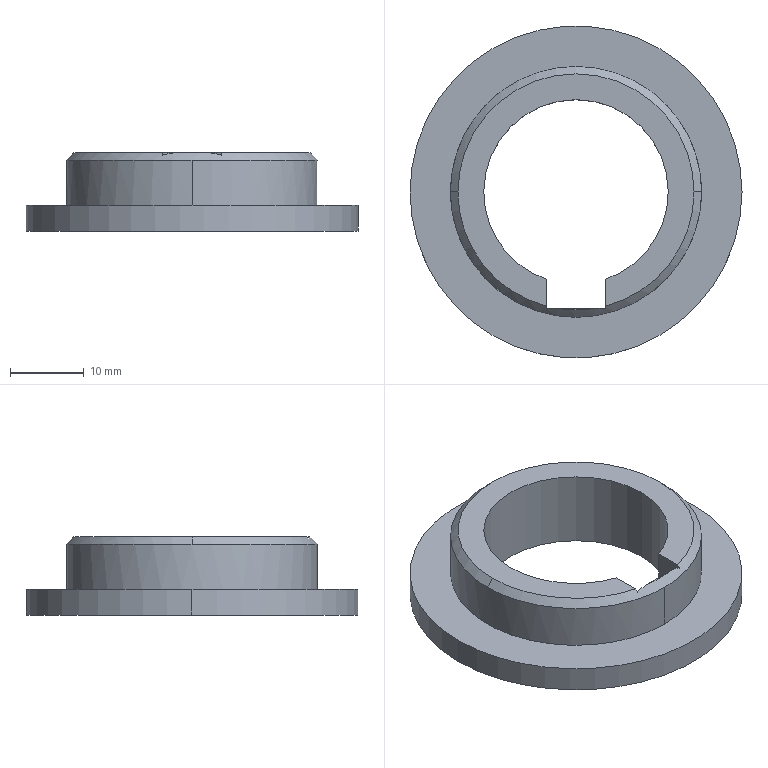Part | NX | 1 solid | 16 faces | box 45 x 45 x 10.6 mm | volume 6459 mm3 | plane 7 | cylinder 7 | cone 2 | commonest cylinder face diameters 25 x3 34 x2 45 x2
STEP:
#1=CARTESIAN_POINT('',(22.5,0.,0.));
#2=VERTEX_POINT('',#1);
#3=CARTESIAN_POINT('',(-22.5,0.,0.));
#4=VERTEX_POINT('',#3);
#5=CARTESIAN_POINT('',(0.,0.,0.));
#6=DIRECTION('',(0.,0.,1.));
#7=DIRECTION('',(-1.,0.,0.));
#8=AXIS2_PLACEMENT_3D('',#5,#6,#7);
#9=CIRCLE('',#8,22.5);
#10=EDGE_CURVE('',#2,#4,#9,.T.);
#11=ORIENTED_EDGE('',*,*,#10,.F.);
#12=CARTESIAN_POINT('',(0.,0.,0.));
#13=DIRECTION('',(0.,0.,1.));
#14=DIRECTION('',(-1.,0.,0.));
#15=AXIS2_PLACEMENT_3D('',#12,#13,#14);
#16=CIRCLE('',#15,22.5);
#17=EDGE_CURVE('',#4,#2,#16,.T.);
#18=ORIENTED_EDGE('',*,*,#17,.F.);
#19=EDGE_LOOP('',(#11,#18));
#20=FACE_BOUND('',#19,.T.);
#21=CARTESIAN_POINT('',(-4.,-11.843,0.));
#22=VERTEX_POINT('',#21);
#23=CARTESIAN_POINT('',(-12.5,0.,0.));
#24=VERTEX_POINT('',#23);
#25=CARTESIAN_POINT('',(0.,0.,0.));
#26=DIRECTION('',(0.,0.,-1.));
#27=DIRECTION('',(1.,0.,0.));
#28=AXIS2_PLACEMENT_3D('',#25,#26,#27);
#29=CIRCLE('',#28,12.5);
#30=EDGE_CURVE('',#22,#24,#29,.T.);
#31=ORIENTED_EDGE('',*,*,#30,.F.);
#32=CARTESIAN_POINT('',(-4.,-15.8,0.));
#33=VERTEX_POINT('',#32);
#34=CARTESIAN_POINT('',(-4.,0.,0.));
#35=DIRECTION('',(0.,-1.,0.));
#36=VECTOR('',#35,1000.);
#37=LINE('',#34,#36);
#38=EDGE_CURVE('',#22,#33,#37,.T.);
#39=ORIENTED_EDGE('',*,*,#38,.T.);
#40=CARTESIAN_POINT('',(4.,-15.8,0.));
#41=VERTEX_POINT('',#40);
#42=CARTESIAN_POINT('',(0.,-15.8,0.));
#43=DIRECTION('',(1.,0.,0.));
#44=VECTOR('',#43,1000.);
#45=LINE('',#42,#44);
#46=EDGE_CURVE('',#33,#41,#45,.T.);
#47=ORIENTED_EDGE('',*,*,#46,.T.);
#48=CARTESIAN_POINT('',(4.,-11.843,0.));
#49=VERTEX_POINT('',#48);
#50=CARTESIAN_POINT('',(4.,0.,0.));
#51=DIRECTION('',(0.,1.,0.));
#52=VECTOR('',#51,1000.);
#53=LINE('',#50,#52);
#54=EDGE_CURVE('',#41,#49,#53,.T.);
#55=ORIENTED_EDGE('',*,*,#54,.T.);
#56=CARTESIAN_POINT('',(12.5,0.,0.));
#57=VERTEX_POINT('',#56);
#58=CARTESIAN_POINT('',(0.,0.,0.));
#59=DIRECTION('',(0.,0.,-1.));
#60=DIRECTION('',(1.,0.,0.));
#61=AXIS2_PLACEMENT_3D('',#58,#59,#60);
#62=CIRCLE('',#61,12.5);
#63=EDGE_CURVE('',#57,#49,#62,.T.);
#64=ORIENTED_EDGE('',*,*,#63,.F.);
#65=CARTESIAN_POINT('',(0.,0.,0.));
#66=DIRECTION('',(0.,0.,-1.));
#67=DIRECTION('',(1.,0.,0.));
#68=AXIS2_PLACEMENT_3D('',#65,#66,#67);
#69=CIRCLE('',#68,12.5);
#70=EDGE_CURVE('',#24,#57,#69,.T.);
#71=ORIENTED_EDGE('',*,*,#70,.F.);
#72=EDGE_LOOP('',(#31,#39,#47,#55,#64,#71));
#73=FACE_BOUND('',#72,.T.);
#74=CARTESIAN_POINT('',(0.,0.,0.));
#75=DIRECTION('',(0.,0.,1.));
#76=DIRECTION('',(1.,0.,0.));
#77=AXIS2_PLACEMENT_3D('',#74,#75,#76);
#78=PLANE('',#77);
#79=ADVANCED_FACE('',(#20,#73),#78,.F.);
#80=ORIENTED_EDGE('',*,*,#10,.T.);
#81=CARTESIAN_POINT('',(-22.5,0.,3.5));
#82=VERTEX_POINT('',#81);
#83=CARTESIAN_POINT('',(-22.5,0.,0.));
#84=DIRECTION('',(0.,0.,1.));
#85=VECTOR('',#84,1000.);
#86=LINE('',#83,#85);
#87=EDGE_CURVE('',#82,#4,#86,.F.);
#88=ORIENTED_EDGE('',*,*,#87,.F.);
#89=CARTESIAN_POINT('',(22.5,0.,3.5));
#90=VERTEX_POINT('',#89);
#91=CARTESIAN_POINT('',(0.,0.,3.5));
#92=DIRECTION('',(0.,0.,1.));
#93=DIRECTION('',(1.,0.,0.));
#94=AXIS2_PLACEMENT_3D('',#91,#92,#93);
#95=CIRCLE('',#94,22.5);
#96=EDGE_CURVE('',#90,#82,#95,.T.);
#97=ORIENTED_EDGE('',*,*,#96,.F.);
#98=CARTESIAN_POINT('',(22.5,0.,0.));
#99=DIRECTION('',(0.,0.,1.));
#100=VECTOR('',#99,1000.);
#101=LINE('',#98,#100);
#102=EDGE_CURVE('',#90,#2,#101,.F.);
#103=ORIENTED_EDGE('',*,*,#102,.T.);
#104=EDGE_LOOP('',(#80,#88,#97,#103));
#105=FACE_BOUND('',#104,.T.);
#106=CARTESIAN_POINT('',(0.,0.,0.));
#107=DIRECTION('',(0.,0.,1.));
#108=DIRECTION('',(1.,0.,0.));
#109=AXIS2_PLACEMENT_3D('',#106,#107,#108);
#110=CYLINDRICAL_SURFACE('',#109,22.5);
#111=ADVANCED_FACE('',(#105),#110,.T.);
#112=CARTESIAN_POINT('',(12.5,0.,10.6));
#113=VERTEX_POINT('',#112);
#114=CARTESIAN_POINT('',(12.5,0.,0.));
#115=DIRECTION('',(0.,0.,1.));
#116=VECTOR('',#115,1000.);
#117=LINE('',#114,#116);
#118=EDGE_CURVE('',#57,#113,#117,.T.);
#119=ORIENTED_EDGE('',*,*,#118,.F.);
#120=ORIENTED_EDGE('',*,*,#63,.T.);
#121=CARTESIAN_POINT('',(4.,-11.843,10.6));
#122=VERTEX_POINT('',#121);
#123=CARTESIAN_POINT('',(4.,-11.843,0.));
#124=DIRECTION('',(0.,0.,1.));
#125=VECTOR('',#124,1000.);
#126=LINE('',#123,#125);
#127=EDGE_CURVE('',#49,#122,#126,.T.);
#128=ORIENTED_EDGE('',*,*,#127,.T.);
#129=CARTESIAN_POINT('',(0.,0.,10.6));
#130=DIRECTION('',(0.,0.,-1.));
#131=DIRECTION('',(1.,0.,0.));
#132=AXIS2_PLACEMENT_3D('',#129,#130,#131);
#133=CIRCLE('',#132,12.5);
#134=EDGE_CURVE('',#113,#122,#133,.T.);
#135=ORIENTED_EDGE('',*,*,#134,.F.);
#136=EDGE_LOOP('',(#119,#120,#128,#135));
#137=FACE_BOUND('',#136,.T.);
#138=CARTESIAN_POINT('',(0.,0.,0.));
#139=DIRECTION('',(0.,0.,1.));
#140=DIRECTION('',(1.,0.,0.));
#141=AXIS2_PLACEMENT_3D('',#138,#139,#140);
#142=CYLINDRICAL_SURFACE('',#141,12.5);
#143=ADVANCED_FACE('',(#137),#142,.F.);
#144=CARTESIAN_POINT('',(0.,0.,3.5));
#145=DIRECTION('',(0.,0.,1.));
#146=DIRECTION('',(1.,0.,0.));
#147=AXIS2_PLACEMENT_3D('',#144,#145,#146);
#148=CIRCLE('',#147,22.5);
#149=EDGE_CURVE('',#82,#90,#148,.T.);
#150=ORIENTED_EDGE('',*,*,#149,.T.);
#151=ORIENTED_EDGE('',*,*,#96,.T.);
#152=EDGE_LOOP('',(#150,#151));
#153=FACE_BOUND('',#152,.T.);
#154=CARTESIAN_POINT('',(0.,17.,3.5));
#155=VERTEX_POINT('',#154);
#156=CARTESIAN_POINT('',(0.,-17.,3.5));
#157=VERTEX_POINT('',#156);
#158=CARTESIAN_POINT('',(0.,0.,3.5));
#159=DIRECTION('',(0.,0.,1.));
#160=DIRECTION('',(0.,-1.,0.));
#161=AXIS2_PLACEMENT_3D('',#158,#159,#160);
#162=CIRCLE('',#161,17.);
#163=EDGE_CURVE('',#155,#157,#162,.T.);
#164=ORIENTED_EDGE('',*,*,#163,.F.);
#165=CARTESIAN_POINT('',(0.,0.,3.5));
#166=DIRECTION('',(0.,0.,1.));
#167=DIRECTION('',(0.,-1.,0.));
#168=AXIS2_PLACEMENT_3D('',#165,#166,#167);
#169=CIRCLE('',#168,17.);
#170=EDGE_CURVE('',#157,#155,#169,.T.);
#171=ORIENTED_EDGE('',*,*,#170,.F.);
#172=EDGE_LOOP('',(#164,#171));
#173=FACE_BOUND('',#172,.T.);
#174=CARTESIAN_POINT('',(0.,0.,3.5));
#175=DIRECTION('',(0.,0.,1.));
#176=DIRECTION('',(1.,0.,0.));
#177=AXIS2_PLACEMENT_3D('',#174,#175,#176);
#178=PLANE('',#177);
#179=ADVANCED_FACE('',(#153,#173),#178,.T.);
#180=CARTESIAN_POINT('',(-17.,0.,9.6));
#181=VERTEX_POINT('',#180);
#182=CARTESIAN_POINT('',(0.,17.,9.6));
#183=VERTEX_POINT('',#182);
#184=CARTESIAN_POINT('',(0.,0.,9.6));
#185=DIRECTION('',(0.,0.,-1.));
#186=DIRECTION('',(-1.,0.,0.));
#187=AXIS2_PLACEMENT_3D('',#184,#185,#186);
#188=CIRCLE('',#187,17.);
#189=EDGE_CURVE('',#181,#183,#188,.T.);
#190=ORIENTED_EDGE('',*,*,#189,.T.);
#191=CARTESIAN_POINT('',(0.,17.,3.5));
#192=DIRECTION('',(0.,0.,1.));
#193=VECTOR('',#192,1000.);
#194=LINE('',#191,#193);
#195=EDGE_CURVE('',#155,#183,#194,.T.);
#196=ORIENTED_EDGE('',*,*,#195,.F.);
#197=ORIENTED_EDGE('',*,*,#163,.T.);
#198=CARTESIAN_POINT('',(0.,-17.,9.6));
#199=VERTEX_POINT('',#198);
#200=CARTESIAN_POINT('',(0.,-17.,3.5));
#201=DIRECTION('',(0.,0.,1.));
#202=VECTOR('',#201,1000.);
#203=LINE('',#200,#202);
#204=EDGE_CURVE('',#157,#199,#203,.T.);
#205=ORIENTED_EDGE('',*,*,#204,.T.);
#206=CARTESIAN_POINT('',(0.,0.,9.6));
#207=DIRECTION('',(0.,0.,-1.));
#208=DIRECTION('',(-1.,0.,0.));
#209=AXIS2_PLACEMENT_3D('',#206,#207,#208);
#210=CIRCLE('',#209,17.);
#211=EDGE_CURVE('',#199,#181,#210,.T.);
#212=ORIENTED_EDGE('',*,*,#211,.T.);
#213=EDGE_LOOP('',(#190,#196,#197,#205,#212));
#214=FACE_BOUND('',#213,.T.);
#215=CARTESIAN_POINT('',(0.,0.,3.5));
#216=DIRECTION('',(0.,0.,1.));
#217=DIRECTION('',(0.,-1.,0.));
#218=AXIS2_PLACEMENT_3D('',#215,#216,#217);
#219=CYLINDRICAL_SURFACE('',#218,17.);
#220=ADVANCED_FACE('',(#214),#219,.T.);
#221=CARTESIAN_POINT('',(16.,0.,10.6));
#222=VERTEX_POINT('',#221);
#223=CARTESIAN_POINT('',(4.,-15.492,10.6));
#224=VERTEX_POINT('',#223);
#225=CARTESIAN_POINT('',(0.,0.,10.6));
#226=DIRECTION('',(0.,0.,-1.));
#227=DIRECTION('',(-1.,0.,0.));
#228=AXIS2_PLACEMENT_3D('',#225,#226,#227);
#229=CIRCLE('',#228,16.);
#230=EDGE_CURVE('',#222,#224,#229,.T.);
#231=ORIENTED_EDGE('',*,*,#230,.F.);
#232=CARTESIAN_POINT('',(-16.,0.,10.6));
#233=VERTEX_POINT('',#232);
#234=CARTESIAN_POINT('',(0.,0.,10.6));
#235=DIRECTION('',(0.,0.,-1.));
#236=DIRECTION('',(-1.,0.,0.));
#237=AXIS2_PLACEMENT_3D('',#234,#235,#236);
#238=CIRCLE('',#237,16.);
#239=EDGE_CURVE('',#233,#222,#238,.T.);
#240=ORIENTED_EDGE('',*,*,#239,.F.);
#241=CARTESIAN_POINT('',(-4.,-15.492,10.6));
#242=VERTEX_POINT('',#241);
#243=CARTESIAN_POINT('',(0.,0.,10.6));
#244=DIRECTION('',(0.,0.,-1.));
#245=DIRECTION('',(-1.,0.,0.));
#246=AXIS2_PLACEMENT_3D('',#243,#244,#245);
#247=CIRCLE('',#246,16.);
#248=EDGE_CURVE('',#242,#233,#247,.T.);
#249=ORIENTED_EDGE('',*,*,#248,.F.);
#250=CARTESIAN_POINT('',(-4.,-11.843,10.6));
#251=VERTEX_POINT('',#250);
#252=CARTESIAN_POINT('',(-4.,0.,10.6));
#253=DIRECTION('',(0.,-1.,0.));
#254=VECTOR('',#253,1000.);
#255=LINE('',#252,#254);
#256=EDGE_CURVE('',#251,#242,#255,.T.);
#257=ORIENTED_EDGE('',*,*,#256,.F.);
#258=CARTESIAN_POINT('',(-12.5,0.,10.6));
#259=VERTEX_POINT('',#258);
#260=CARTESIAN_POINT('',(0.,0.,10.6));
#261=DIRECTION('',(0.,0.,-1.));
#262=DIRECTION('',(1.,0.,0.));
#263=AXIS2_PLACEMENT_3D('',#260,#261,#262);
#264=CIRCLE('',#263,12.5);
#265=EDGE_CURVE('',#251,#259,#264,.T.);
#266=ORIENTED_EDGE('',*,*,#265,.T.);
#267=CARTESIAN_POINT('',(0.,0.,10.6));
#268=DIRECTION('',(0.,0.,-1.));
#269=DIRECTION('',(1.,0.,0.));
#270=AXIS2_PLACEMENT_3D('',#267,#268,#269);
#271=CIRCLE('',#270,12.5);
#272=EDGE_CURVE('',#259,#113,#271,.T.);
#273=ORIENTED_EDGE('',*,*,#272,.T.);
#274=ORIENTED_EDGE('',*,*,#134,.T.);
#275=CARTESIAN_POINT('',(4.,0.,10.6));
#276=DIRECTION('',(0.,1.,0.));
#277=VECTOR('',#276,1000.);
#278=LINE('',#275,#277);
#279=EDGE_CURVE('',#224,#122,#278,.T.);
#280=ORIENTED_EDGE('',*,*,#279,.F.);
#281=EDGE_LOOP('',(#231,#240,#249,#257,#266,#273,#274,#280));
#282=FACE_BOUND('',#281,.T.);
#283=CARTESIAN_POINT('',(14.369,-9.107,10.6));
#284=DIRECTION('',(0.,0.,1.));
#285=DIRECTION('',(1.,0.,0.));
#286=AXIS2_PLACEMENT_3D('',#283,#284,#285);
#287=PLANE('',#286);
#288=ADVANCED_FACE('',(#282),#287,.T.);
#289=ORIENTED_EDGE('',*,*,#189,.F.);
#290=CARTESIAN_POINT('',(-16.,0.,10.6));
#291=DIRECTION('',(-0.7071,0.,-0.7071));
#292=VECTOR('',#291,1000.);
#293=LINE('',#290,#292);
#294=EDGE_CURVE('',#181,#233,#293,.F.);
#295=ORIENTED_EDGE('',*,*,#294,.T.);
#296=ORIENTED_EDGE('',*,*,#239,.T.);
#297=CARTESIAN_POINT('',(17.,0.,9.6));
#298=VERTEX_POINT('',#297);
#299=CARTESIAN_POINT('',(16.,0.,10.6));
#300=DIRECTION('',(0.7071,0.,-0.7071));
#301=VECTOR('',#300,1000.);
#302=LINE('',#299,#301);
#303=EDGE_CURVE('',#298,#222,#302,.F.);
#304=ORIENTED_EDGE('',*,*,#303,.F.);
#305=CARTESIAN_POINT('',(0.,0.,9.6));
#306=DIRECTION('',(0.,0.,-1.));
#307=DIRECTION('',(-1.,0.,0.));
#308=AXIS2_PLACEMENT_3D('',#305,#306,#307);
#309=CIRCLE('',#308,17.);
#310=EDGE_CURVE('',#183,#298,#309,.T.);
#311=ORIENTED_EDGE('',*,*,#310,.F.);
#312=EDGE_LOOP('',(#289,#295,#296,#304,#311));
#313=FACE_BOUND('',#312,.T.);
#314=CARTESIAN_POINT('',(0.,0.,10.6));
#315=DIRECTION('',(0.,0.,-1.));
#316=DIRECTION('',(-1.,0.,0.));
#317=AXIS2_PLACEMENT_3D('',#314,#315,#316);
#318=CONICAL_SURFACE('',#317,16.,0.7854);
#319=ADVANCED_FACE('',(#313),#318,.T.);
#320=CARTESIAN_POINT('',(-2.522,-15.8,10.6));
#321=VERTEX_POINT('',#320);
#322=CARTESIAN_POINT('',(2.522,-15.8,10.6));
#323=VERTEX_POINT('',#322);
#324=CARTESIAN_POINT('',(0.,-15.8,10.6));
#325=DIRECTION('',(1.,0.,0.));
#326=VECTOR('',#325,1000.);
#327=LINE('',#324,#326);
#328=EDGE_CURVE('',#321,#323,#327,.T.);
#329=ORIENTED_EDGE('',*,*,#328,.F.);
#330=CARTESIAN_POINT('',(0.,0.,10.6));
#331=DIRECTION('',(0.,0.,-1.));
#332=DIRECTION('',(-1.,0.,0.));
#333=AXIS2_PLACEMENT_3D('',#330,#331,#332);
#334=CIRCLE('',#333,16.);
#335=EDGE_CURVE('',#323,#321,#334,.T.);
#336=ORIENTED_EDGE('',*,*,#335,.F.);
#337=EDGE_LOOP('',(#329,#336));
#338=FACE_BOUND('',#337,.T.);
#339=CARTESIAN_POINT('',(14.369,-9.107,10.6));
#340=DIRECTION('',(0.,0.,1.));
#341=DIRECTION('',(1.,0.,0.));
#342=AXIS2_PLACEMENT_3D('',#339,#340,#341);
#343=PLANE('',#342);
#344=ADVANCED_FACE('',(#338),#343,.T.);
#345=CARTESIAN_POINT('',(-4.,-15.8,10.302));
#346=VERTEX_POINT('',#345);
#347=CARTESIAN_POINT('',(-4.,-15.8,10.302));
#348=CARTESIAN_POINT('',(-3.878,-15.8,10.331));
#349=CARTESIAN_POINT('',(-3.756,-15.8,10.36));
#350=CARTESIAN_POINT('',(-3.634,-15.8,10.388));
#351=CARTESIAN_POINT('',(-3.511,-15.8,10.415));
#352=CARTESIAN_POINT('',(-3.389,-15.8,10.441));
#353=CARTESIAN_POINT('',(-3.265,-15.8,10.466));
#354=CARTESIAN_POINT('',(-3.142,-15.8,10.491));
#355=CARTESIAN_POINT('',(-3.019,-15.8,10.515));
#356=CARTESIAN_POINT('',(-2.895,-15.8,10.537));
#357=CARTESIAN_POINT('',(-2.771,-15.8,10.559));
#358=CARTESIAN_POINT('',(-2.646,-15.8,10.58));
#359=CARTESIAN_POINT('',(-2.522,-15.8,10.6));
#360=B_SPLINE_CURVE_WITH_KNOTS('',3,(#347,#348,#349,#350,#351,#352,#353,#354,#355,#356,#357,#358,#359),.UNSPECIFIED.,.F.,.F.,(4,3,3,3,4),(0.,0.3761,0.7528,1.13,1.508),.UNSPECIFIED.);
#361=EDGE_CURVE('',#346,#321,#360,.T.);
#362=ORIENTED_EDGE('',*,*,#361,.T.);
#363=ORIENTED_EDGE('',*,*,#328,.T.);
#364=CARTESIAN_POINT('',(4.,-15.8,10.302));
#365=VERTEX_POINT('',#364);
#366=CARTESIAN_POINT('',(2.522,-15.8,10.6));
#367=CARTESIAN_POINT('',(2.646,-15.8,10.58));
#368=CARTESIAN_POINT('',(2.77,-15.8,10.56));
#369=CARTESIAN_POINT('',(2.893,-15.8,10.537));
#370=CARTESIAN_POINT('',(3.017,-15.8,10.515));
#371=CARTESIAN_POINT('',(3.14,-15.8,10.491));
#372=CARTESIAN_POINT('',(3.264,-15.8,10.466));
#373=CARTESIAN_POINT('',(3.387,-15.8,10.442));
#374=CARTESIAN_POINT('',(3.51,-15.8,10.415));
#375=CARTESIAN_POINT('',(3.633,-15.8,10.388));
#376=CARTESIAN_POINT('',(3.755,-15.8,10.36));
#377=CARTESIAN_POINT('',(3.878,-15.8,10.332));
#378=CARTESIAN_POINT('',(4.,-15.8,10.302));
#379=B_SPLINE_CURVE_WITH_KNOTS('',3,(#366,#367,#368,#369,#370,#371,#372,#373,#374,#375,#376,#377,#378),.UNSPECIFIED.,.F.,.F.,(4,3,3,3,4),(0.,0.3767,0.7537,1.131,1.508),.UNSPECIFIED.);
#380=EDGE_CURVE('',#323,#365,#379,.T.);
#381=ORIENTED_EDGE('',*,*,#380,.T.);
#382=CARTESIAN_POINT('',(4.,-15.8,11.66));
#383=DIRECTION('',(0.,0.,-1.));
#384=VECTOR('',#383,1000.);
#385=LINE('',#382,#384);
#386=EDGE_CURVE('',#365,#41,#385,.T.);
#387=ORIENTED_EDGE('',*,*,#386,.T.);
#388=ORIENTED_EDGE('',*,*,#46,.F.);
#389=CARTESIAN_POINT('',(-4.,-15.8,11.66));
#390=DIRECTION('',(0.,0.,-1.));
#391=VECTOR('',#390,1000.);
#392=LINE('',#389,#391);
#393=EDGE_CURVE('',#346,#33,#392,.T.);
#394=ORIENTED_EDGE('',*,*,#393,.F.);
#395=EDGE_LOOP('',(#362,#363,#381,#387,#388,#394));
#396=FACE_BOUND('',#395,.T.);
#397=CARTESIAN_POINT('',(-4.,-15.8,11.66));
#398=DIRECTION('',(0.,-1.,0.));
#399=DIRECTION('',(0.,0.,-1.));
#400=AXIS2_PLACEMENT_3D('',#397,#398,#399);
#401=PLANE('',#400);
#402=ADVANCED_FACE('',(#396),#401,.F.);
#403=ORIENTED_EDGE('',*,*,#54,.F.);
#404=ORIENTED_EDGE('',*,*,#386,.F.);
#405=CARTESIAN_POINT('',(4.,-15.8,10.302));
#406=CARTESIAN_POINT('',(4.,-15.774,10.326));
#407=CARTESIAN_POINT('',(4.,-15.749,10.351));
#408=CARTESIAN_POINT('',(4.,-15.723,10.376));
#409=CARTESIAN_POINT('',(4.,-15.697,10.401));
#410=CARTESIAN_POINT('',(4.,-15.672,10.426));
#411=CARTESIAN_POINT('',(4.,-15.646,10.451));
#412=CARTESIAN_POINT('',(4.,-15.62,10.476));
#413=CARTESIAN_POINT('',(4.,-15.595,10.501));
#414=CARTESIAN_POINT('',(4.,-15.569,10.525));
#415=CARTESIAN_POINT('',(4.,-15.543,10.55));
#416=CARTESIAN_POINT('',(4.,-15.518,10.575));
#417=CARTESIAN_POINT('',(4.,-15.492,10.6));
#418=B_SPLINE_CURVE_WITH_KNOTS('',3,(#405,#406,#407,#408,#409,#410,#411,#412,#413,#414,#415,#416,#417),.UNSPECIFIED.,.F.,.F.,(4,3,3,3,4),(0.,0.1072,0.2145,0.3217,0.4289),.UNSPECIFIED.);
#419=EDGE_CURVE('',#365,#224,#418,.T.);
#420=ORIENTED_EDGE('',*,*,#419,.T.);
#421=ORIENTED_EDGE('',*,*,#279,.T.);
#422=ORIENTED_EDGE('',*,*,#127,.F.);
#423=EDGE_LOOP('',(#403,#404,#420,#421,#422));
#424=FACE_BOUND('',#423,.T.);
#425=CARTESIAN_POINT('',(4.,-15.8,11.66));
#426=DIRECTION('',(1.,0.,0.));
#427=DIRECTION('',(0.,1.,0.));
#428=AXIS2_PLACEMENT_3D('',#425,#426,#427);
#429=PLANE('',#428);
#430=ADVANCED_FACE('',(#424),#429,.F.);
#431=ORIENTED_EDGE('',*,*,#256,.T.);
#432=CARTESIAN_POINT('',(-4.,-15.492,10.6));
#433=CARTESIAN_POINT('',(-4.,-15.518,10.575));
#434=CARTESIAN_POINT('',(-4.,-15.543,10.55));
#435=CARTESIAN_POINT('',(-4.,-15.569,10.525));
#436=CARTESIAN_POINT('',(-4.,-15.595,10.501));
#437=CARTESIAN_POINT('',(-4.,-15.62,10.476));
#438=CARTESIAN_POINT('',(-4.,-15.646,10.451));
#439=CARTESIAN_POINT('',(-4.,-15.672,10.426));
#440=CARTESIAN_POINT('',(-4.,-15.697,10.401));
#441=CARTESIAN_POINT('',(-4.,-15.723,10.376));
#442=CARTESIAN_POINT('',(-4.,-15.749,10.351));
#443=CARTESIAN_POINT('',(-4.,-15.774,10.326));
#444=CARTESIAN_POINT('',(-4.,-15.8,10.302));
#445=B_SPLINE_CURVE_WITH_KNOTS('',3,(#432,#433,#434,#435,#436,#437,#438,#439,#440,#441,#442,#443,#444),.UNSPECIFIED.,.F.,.F.,(4,3,3,3,4),(0.,0.1072,0.2145,0.3217,0.4289),.UNSPECIFIED.);
#446=EDGE_CURVE('',#242,#346,#445,.T.);
#447=ORIENTED_EDGE('',*,*,#446,.T.);
#448=ORIENTED_EDGE('',*,*,#393,.T.);
#449=ORIENTED_EDGE('',*,*,#38,.F.);
#450=CARTESIAN_POINT('',(-4.,-11.843,0.));
#451=DIRECTION('',(0.,0.,1.));
#452=VECTOR('',#451,1000.);
#453=LINE('',#450,#452);
#454=EDGE_CURVE('',#22,#251,#453,.T.);
#455=ORIENTED_EDGE('',*,*,#454,.T.);
#456=EDGE_LOOP('',(#431,#447,#448,#449,#455));
#457=FACE_BOUND('',#456,.T.);
#458=CARTESIAN_POINT('',(-4.,-11.843,11.66));
#459=DIRECTION('',(-1.,0.,0.));
#460=DIRECTION('',(0.,0.,1.));
#461=AXIS2_PLACEMENT_3D('',#458,#459,#460);
#462=PLANE('',#461);
#463=ADVANCED_FACE('',(#457),#462,.F.);
#464=ORIENTED_EDGE('',*,*,#230,.T.);
#465=ORIENTED_EDGE('',*,*,#419,.F.);
#466=ORIENTED_EDGE('',*,*,#380,.F.);
#467=ORIENTED_EDGE('',*,*,#335,.T.);
#468=ORIENTED_EDGE('',*,*,#361,.F.);
#469=ORIENTED_EDGE('',*,*,#446,.F.);
#470=ORIENTED_EDGE('',*,*,#248,.T.);
#471=ORIENTED_EDGE('',*,*,#294,.F.);
#472=ORIENTED_EDGE('',*,*,#211,.F.);
#473=CARTESIAN_POINT('',(0.,0.,9.6));
#474=DIRECTION('',(0.,0.,-1.));
#475=DIRECTION('',(-1.,0.,0.));
#476=AXIS2_PLACEMENT_3D('',#473,#474,#475);
#477=CIRCLE('',#476,17.);
#478=EDGE_CURVE('',#298,#199,#477,.T.);
#479=ORIENTED_EDGE('',*,*,#478,.F.);
#480=ORIENTED_EDGE('',*,*,#303,.T.);
#481=EDGE_LOOP('',(#464,#465,#466,#467,#468,#469,#470,#471,#472,#479,#480));
#482=FACE_BOUND('',#481,.T.);
#483=CARTESIAN_POINT('',(0.,0.,10.6));
#484=DIRECTION('',(0.,0.,-1.));
#485=DIRECTION('',(-1.,0.,0.));
#486=AXIS2_PLACEMENT_3D('',#483,#484,#485);
#487=CONICAL_SURFACE('',#486,16.,0.7854);
#488=ADVANCED_FACE('',(#482),#487,.T.);
#489=ORIENTED_EDGE('',*,*,#195,.T.);
#490=ORIENTED_EDGE('',*,*,#310,.T.);
#491=ORIENTED_EDGE('',*,*,#478,.T.);
#492=ORIENTED_EDGE('',*,*,#204,.F.);
#493=ORIENTED_EDGE('',*,*,#170,.T.);
#494=EDGE_LOOP('',(#489,#490,#491,#492,#493));
#495=FACE_BOUND('',#494,.T.);
#496=CARTESIAN_POINT('',(0.,0.,3.5));
#497=DIRECTION('',(0.,0.,1.));
#498=DIRECTION('',(0.,-1.,0.));
#499=AXIS2_PLACEMENT_3D('',#496,#497,#498);
#500=CYLINDRICAL_SURFACE('',#499,17.);
#501=ADVANCED_FACE('',(#495),#500,.T.);
#502=ORIENTED_EDGE('',*,*,#149,.F.);
#503=ORIENTED_EDGE('',*,*,#87,.T.);
#504=ORIENTED_EDGE('',*,*,#17,.T.);
#505=ORIENTED_EDGE('',*,*,#102,.F.);
#506=EDGE_LOOP('',(#502,#503,#504,#505));
#507=FACE_BOUND('',#506,.T.);
#508=CARTESIAN_POINT('',(0.,0.,0.));
#509=DIRECTION('',(0.,0.,1.));
#510=DIRECTION('',(1.,0.,0.));
#511=AXIS2_PLACEMENT_3D('',#508,#509,#510);
#512=CYLINDRICAL_SURFACE('',#511,22.5);
#513=ADVANCED_FACE('',(#507),#512,.T.);
#514=CARTESIAN_POINT('',(-12.5,0.,0.));
#515=DIRECTION('',(0.,0.,1.));
#516=VECTOR('',#515,1000.);
#517=LINE('',#514,#516);
#518=EDGE_CURVE('',#24,#259,#517,.T.);
#519=ORIENTED_EDGE('',*,*,#518,.F.);
#520=ORIENTED_EDGE('',*,*,#70,.T.);
#521=ORIENTED_EDGE('',*,*,#118,.T.);
#522=ORIENTED_EDGE('',*,*,#272,.F.);
#523=EDGE_LOOP('',(#519,#520,#521,#522));
#524=FACE_BOUND('',#523,.T.);
#525=CARTESIAN_POINT('',(0.,0.,0.));
#526=DIRECTION('',(0.,0.,1.));
#527=DIRECTION('',(1.,0.,0.));
#528=AXIS2_PLACEMENT_3D('',#525,#526,#527);
#529=CYLINDRICAL_SURFACE('',#528,12.5);
#530=ADVANCED_FACE('',(#524),#529,.F.);
#531=ORIENTED_EDGE('',*,*,#30,.T.);
#532=ORIENTED_EDGE('',*,*,#518,.T.);
#533=ORIENTED_EDGE('',*,*,#265,.F.);
#534=ORIENTED_EDGE('',*,*,#454,.F.);
#535=EDGE_LOOP('',(#531,#532,#533,#534));
#536=FACE_BOUND('',#535,.T.);
#537=CARTESIAN_POINT('',(0.,0.,0.));
#538=DIRECTION('',(0.,0.,1.));
#539=DIRECTION('',(1.,0.,0.));
#540=AXIS2_PLACEMENT_3D('',#537,#538,#539);
#541=CYLINDRICAL_SURFACE('',#540,12.5);
#542=ADVANCED_FACE('',(#536),#541,.F.);
#543=CLOSED_SHELL('',(#79,#111,#143,#179,#220,#288,#319,#344,#402,#430,#463,#488,#501,#513,#530,#542));
#544=MANIFOLD_SOLID_BREP('',#543);
#545=(LENGTH_UNIT()NAMED_UNIT(*)SI_UNIT(.MILLI.,.METRE.));
#546=UNCERTAINTY_MEASURE_WITH_UNIT(LENGTH_MEASURE(0.00001),#545,'','');
#547=(NAMED_UNIT(*)PLANE_ANGLE_UNIT()SI_UNIT($,.RADIAN.));
#548=(NAMED_UNIT(*)SI_UNIT($,.STERADIAN.)SOLID_ANGLE_UNIT());
#549=(GEOMETRIC_REPRESENTATION_CONTEXT(3)GLOBAL_UNCERTAINTY_ASSIGNED_CONTEXT((#546))GLOBAL_UNIT_ASSIGNED_CONTEXT((#545,#547,#548))REPRESENTATION_CONTEXT('',''));
#550=ADVANCED_BREP_SHAPE_REPRESENTATION('',(#544),#549);